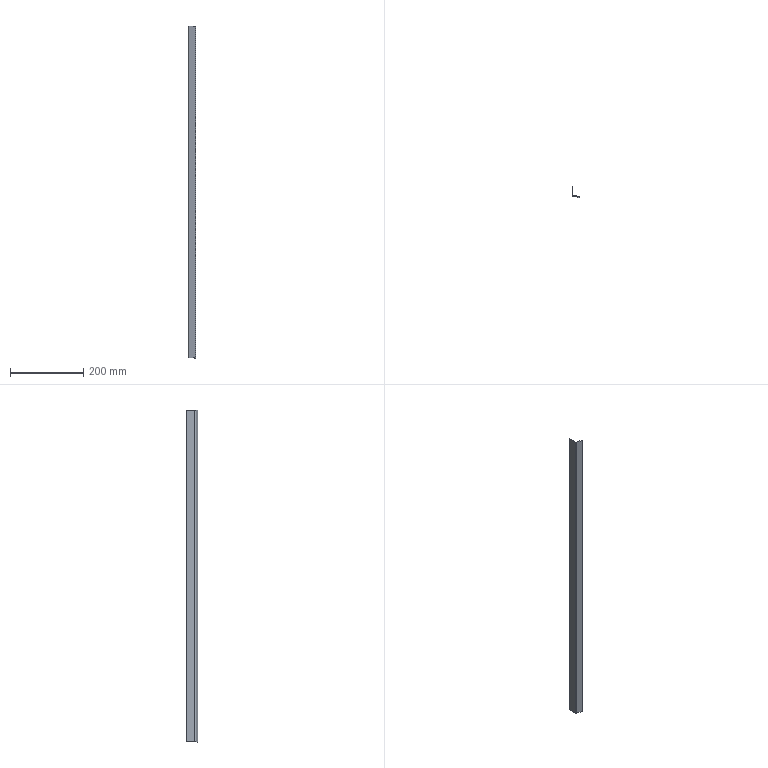Part | STEP file | 750078467 | 1 solid | 10 faces | box 19.629 x 30.176 x 903.6 mm | volume 47356 mm3 | plane 8 | cylinder 2 | commonest cylinder face diameters 2.4 x1 4.8 x1
STEP:
#1=CARTESIAN_POINT('',(0.,1.842,451.8));
#2=VERTEX_POINT('',#1);
#3=CARTESIAN_POINT('',(0.,25.,451.8));
#4=VERTEX_POINT('',#3);
#5=CARTESIAN_POINT('',(0.,0.,451.8));
#6=DIRECTION('',(0.,1.,0.));
#7=VECTOR('',#6,1000.);
#8=LINE('',#5,#7);
#9=EDGE_CURVE('',#2,#4,#8,.T.);
#10=ORIENTED_EDGE('',*,*,#9,.T.);
#11=CARTESIAN_POINT('',(0.,25.,-451.8));
#12=VERTEX_POINT('',#11);
#13=CARTESIAN_POINT('',(0.,25.,451.8));
#14=DIRECTION('',(0.,0.,-1.));
#15=VECTOR('',#14,1000.);
#16=LINE('',#13,#15);
#17=EDGE_CURVE('',#4,#12,#16,.T.);
#18=ORIENTED_EDGE('',*,*,#17,.T.);
#19=CARTESIAN_POINT('',(0.,1.842,-451.8));
#20=VERTEX_POINT('',#19);
#21=CARTESIAN_POINT('',(0.,0.,-451.8));
#22=DIRECTION('',(0.,-1.,0.));
#23=VECTOR('',#22,1000.);
#24=LINE('',#21,#23);
#25=EDGE_CURVE('',#12,#20,#24,.T.);
#26=ORIENTED_EDGE('',*,*,#25,.T.);
#27=CARTESIAN_POINT('',(0.,1.842,451.8));
#28=DIRECTION('',(0.,0.,1.));
#29=VECTOR('',#28,1000.);
#30=LINE('',#27,#29);
#31=EDGE_CURVE('',#20,#2,#30,.T.);
#32=ORIENTED_EDGE('',*,*,#31,.T.);
#33=EDGE_LOOP('',(#10,#18,#26,#32));
#34=FACE_OUTER_BOUND('',#33,.T.);
#35=CARTESIAN_POINT('',(0.,0.,451.8));
#36=DIRECTION('',(-1.,0.,0.));
#37=DIRECTION('',(0.,0.,1.));
#38=AXIS2_PLACEMENT_3D('',#35,#36,#37);
#39=PLANE('',#38);
#40=ADVANCED_FACE('',(#34),#39,.T.);
#41=CARTESIAN_POINT('',(1.2,25.,-451.8));
#42=VERTEX_POINT('',#41);
#43=CARTESIAN_POINT('',(0.,25.,-451.8));
#44=DIRECTION('',(-1.,0.,0.));
#45=VECTOR('',#44,1000.);
#46=LINE('',#43,#45);
#47=EDGE_CURVE('',#42,#12,#46,.T.);
#48=ORIENTED_EDGE('',*,*,#47,.T.);
#49=ORIENTED_EDGE('',*,*,#17,.F.);
#50=CARTESIAN_POINT('',(1.2,25.,451.8));
#51=VERTEX_POINT('',#50);
#52=CARTESIAN_POINT('',(0.,25.,451.8));
#53=DIRECTION('',(1.,0.,0.));
#54=VECTOR('',#53,1000.);
#55=LINE('',#52,#54);
#56=EDGE_CURVE('',#4,#51,#55,.T.);
#57=ORIENTED_EDGE('',*,*,#56,.T.);
#58=CARTESIAN_POINT('',(1.2,25.,451.8));
#59=DIRECTION('',(0.,0.,-1.));
#60=VECTOR('',#59,1000.);
#61=LINE('',#58,#60);
#62=EDGE_CURVE('',#51,#42,#61,.T.);
#63=ORIENTED_EDGE('',*,*,#62,.T.);
#64=EDGE_LOOP('',(#48,#49,#57,#63));
#65=FACE_OUTER_BOUND('',#64,.T.);
#66=CARTESIAN_POINT('',(0.,25.,451.8));
#67=DIRECTION('',(0.,1.,0.));
#68=DIRECTION('',(0.,0.,1.));
#69=AXIS2_PLACEMENT_3D('',#66,#67,#68);
#70=PLANE('',#69);
#71=ADVANCED_FACE('',(#65),#70,.T.);
#72=CARTESIAN_POINT('',(1.2,1.842,451.8));
#73=VERTEX_POINT('',#72);
#74=CARTESIAN_POINT('',(1.2,0.,451.8));
#75=DIRECTION('',(0.,1.,0.));
#76=VECTOR('',#75,1000.);
#77=LINE('',#74,#76);
#78=EDGE_CURVE('',#73,#51,#77,.T.);
#79=ORIENTED_EDGE('',*,*,#78,.T.);
#80=ORIENTED_EDGE('',*,*,#56,.F.);
#81=ORIENTED_EDGE('',*,*,#9,.F.);
#82=CARTESIAN_POINT('',(1.779,-0.4766,451.8));
#83=VERTEX_POINT('',#82);
#84=CARTESIAN_POINT('',(2.4,1.842,451.8));
#85=DIRECTION('',(0.,0.,1.));
#86=DIRECTION('',(-1.,0.,0.));
#87=AXIS2_PLACEMENT_3D('',#84,#85,#86);
#88=CIRCLE('',#87,2.4);
#89=EDGE_CURVE('',#2,#83,#88,.T.);
#90=ORIENTED_EDGE('',*,*,#89,.T.);
#91=CARTESIAN_POINT('',(19.319,-5.176,451.8));
#92=VERTEX_POINT('',#91);
#93=CARTESIAN_POINT('',(1.779,-0.4766,451.8));
#94=DIRECTION('',(0.9659,-0.2588,0.));
#95=VECTOR('',#94,1000.);
#96=LINE('',#93,#95);
#97=EDGE_CURVE('',#83,#92,#96,.T.);
#98=ORIENTED_EDGE('',*,*,#97,.T.);
#99=CARTESIAN_POINT('',(19.629,-4.017,451.8));
#100=VERTEX_POINT('',#99);
#101=CARTESIAN_POINT('',(19.319,-5.176,451.8));
#102=DIRECTION('',(0.2588,0.9659,0.));
#103=VECTOR('',#102,1000.);
#104=LINE('',#101,#103);
#105=EDGE_CURVE('',#92,#100,#104,.T.);
#106=ORIENTED_EDGE('',*,*,#105,.T.);
#107=CARTESIAN_POINT('',(2.089,0.6825,451.8));
#108=VERTEX_POINT('',#107);
#109=CARTESIAN_POINT('',(19.629,-4.017,451.8));
#110=DIRECTION('',(-0.9659,0.2588,0.));
#111=VECTOR('',#110,1000.);
#112=LINE('',#109,#111);
#113=EDGE_CURVE('',#100,#108,#112,.T.);
#114=ORIENTED_EDGE('',*,*,#113,.T.);
#115=CARTESIAN_POINT('',(2.4,1.842,451.8));
#116=DIRECTION('',(0.,0.,-1.));
#117=DIRECTION('',(-1.,0.,0.));
#118=AXIS2_PLACEMENT_3D('',#115,#116,#117);
#119=CIRCLE('',#118,1.2);
#120=EDGE_CURVE('',#108,#73,#119,.T.);
#121=ORIENTED_EDGE('',*,*,#120,.T.);
#122=EDGE_LOOP('',(#79,#80,#81,#90,#98,#106,#114,#121));
#123=FACE_OUTER_BOUND('',#122,.T.);
#124=CARTESIAN_POINT('',(0.,0.,451.8));
#125=DIRECTION('',(0.,0.,1.));
#126=DIRECTION('',(1.,0.,0.));
#127=AXIS2_PLACEMENT_3D('',#124,#125,#126);
#128=PLANE('',#127);
#129=ADVANCED_FACE('',(#123),#128,.T.);
#130=ORIENTED_EDGE('',*,*,#89,.F.);
#131=ORIENTED_EDGE('',*,*,#31,.F.);
#132=CARTESIAN_POINT('',(1.779,-0.4766,-451.8));
#133=VERTEX_POINT('',#132);
#134=CARTESIAN_POINT('',(2.4,1.842,-451.8));
#135=DIRECTION('',(0.,0.,1.));
#136=DIRECTION('',(-1.,0.,0.));
#137=AXIS2_PLACEMENT_3D('',#134,#135,#136);
#138=CIRCLE('',#137,2.4);
#139=EDGE_CURVE('',#20,#133,#138,.T.);
#140=ORIENTED_EDGE('',*,*,#139,.T.);
#141=CARTESIAN_POINT('',(1.779,-0.4766,451.8));
#142=DIRECTION('',(0.,0.,1.));
#143=VECTOR('',#142,1000.);
#144=LINE('',#141,#143);
#145=EDGE_CURVE('',#133,#83,#144,.T.);
#146=ORIENTED_EDGE('',*,*,#145,.T.);
#147=EDGE_LOOP('',(#130,#131,#140,#146));
#148=FACE_OUTER_BOUND('',#147,.T.);
#149=CARTESIAN_POINT('',(2.4,1.842,451.8));
#150=DIRECTION('',(0.,0.,-1.));
#151=DIRECTION('',(-1.,0.,0.));
#152=AXIS2_PLACEMENT_3D('',#149,#150,#151);
#153=CYLINDRICAL_SURFACE('',#152,2.4);
#154=ADVANCED_FACE('',(#148),#153,.T.);
#155=ORIENTED_EDGE('',*,*,#139,.F.);
#156=ORIENTED_EDGE('',*,*,#25,.F.);
#157=ORIENTED_EDGE('',*,*,#47,.F.);
#158=CARTESIAN_POINT('',(1.2,1.842,-451.8));
#159=VERTEX_POINT('',#158);
#160=CARTESIAN_POINT('',(1.2,-5.176,-451.8));
#161=DIRECTION('',(0.,1.,0.));
#162=VECTOR('',#161,1000.);
#163=LINE('',#160,#162);
#164=EDGE_CURVE('',#159,#42,#163,.T.);
#165=ORIENTED_EDGE('',*,*,#164,.F.);
#166=CARTESIAN_POINT('',(2.089,0.6825,-451.8));
#167=VERTEX_POINT('',#166);
#168=CARTESIAN_POINT('',(2.4,1.842,-451.8));
#169=DIRECTION('',(0.,0.,1.));
#170=DIRECTION('',(-1.,0.,0.));
#171=AXIS2_PLACEMENT_3D('',#168,#169,#170);
#172=CIRCLE('',#171,1.2);
#173=EDGE_CURVE('',#159,#167,#172,.T.);
#174=ORIENTED_EDGE('',*,*,#173,.T.);
#175=CARTESIAN_POINT('',(19.629,-4.017,-451.8));
#176=VERTEX_POINT('',#175);
#177=CARTESIAN_POINT('',(19.629,-4.017,-451.8));
#178=DIRECTION('',(-0.9659,0.2588,0.));
#179=VECTOR('',#178,1000.);
#180=LINE('',#177,#179);
#181=EDGE_CURVE('',#176,#167,#180,.T.);
#182=ORIENTED_EDGE('',*,*,#181,.F.);
#183=CARTESIAN_POINT('',(19.319,-5.176,-451.8));
#184=VERTEX_POINT('',#183);
#185=CARTESIAN_POINT('',(19.319,-5.176,-451.8));
#186=DIRECTION('',(-0.2588,-0.9659,0.));
#187=VECTOR('',#186,1000.);
#188=LINE('',#185,#187);
#189=EDGE_CURVE('',#176,#184,#188,.T.);
#190=ORIENTED_EDGE('',*,*,#189,.T.);
#191=CARTESIAN_POINT('',(1.779,-0.4766,-451.8));
#192=DIRECTION('',(0.9659,-0.2588,0.));
#193=VECTOR('',#192,1000.);
#194=LINE('',#191,#193);
#195=EDGE_CURVE('',#133,#184,#194,.T.);
#196=ORIENTED_EDGE('',*,*,#195,.F.);
#197=EDGE_LOOP('',(#155,#156,#157,#165,#174,#182,#190,#196));
#198=FACE_OUTER_BOUND('',#197,.T.);
#199=CARTESIAN_POINT('',(19.319,-5.176,-451.8));
#200=DIRECTION('',(0.,0.,1.));
#201=DIRECTION('',(1.,0.,0.));
#202=AXIS2_PLACEMENT_3D('',#199,#200,#201);
#203=PLANE('',#202);
#204=ADVANCED_FACE('',(#198),#203,.F.);
#205=ORIENTED_EDGE('',*,*,#62,.F.);
#206=ORIENTED_EDGE('',*,*,#78,.F.);
#207=CARTESIAN_POINT('',(1.2,1.842,451.8));
#208=DIRECTION('',(0.,0.,1.));
#209=VECTOR('',#208,1000.);
#210=LINE('',#207,#209);
#211=EDGE_CURVE('',#159,#73,#210,.T.);
#212=ORIENTED_EDGE('',*,*,#211,.F.);
#213=ORIENTED_EDGE('',*,*,#164,.T.);
#214=EDGE_LOOP('',(#205,#206,#212,#213));
#215=FACE_OUTER_BOUND('',#214,.T.);
#216=CARTESIAN_POINT('',(1.2,0.,451.8));
#217=DIRECTION('',(-1.,0.,0.));
#218=DIRECTION('',(0.,0.,1.));
#219=AXIS2_PLACEMENT_3D('',#216,#217,#218);
#220=PLANE('',#219);
#221=ADVANCED_FACE('',(#215),#220,.F.);
#222=CARTESIAN_POINT('',(2.089,0.6825,451.8));
#223=DIRECTION('',(0.,0.,-1.));
#224=VECTOR('',#223,1000.);
#225=LINE('',#222,#224);
#226=EDGE_CURVE('',#108,#167,#225,.T.);
#227=ORIENTED_EDGE('',*,*,#226,.F.);
#228=ORIENTED_EDGE('',*,*,#113,.F.);
#229=CARTESIAN_POINT('',(19.629,-4.017,451.8));
#230=DIRECTION('',(0.,0.,1.));
#231=VECTOR('',#230,1000.);
#232=LINE('',#229,#231);
#233=EDGE_CURVE('',#176,#100,#232,.T.);
#234=ORIENTED_EDGE('',*,*,#233,.F.);
#235=ORIENTED_EDGE('',*,*,#181,.T.);
#236=EDGE_LOOP('',(#227,#228,#234,#235));
#237=FACE_OUTER_BOUND('',#236,.T.);
#238=CARTESIAN_POINT('',(19.629,-4.017,451.8));
#239=DIRECTION('',(-0.2588,-0.9659,0.));
#240=DIRECTION('',(0.9659,-0.2588,0.));
#241=AXIS2_PLACEMENT_3D('',#238,#239,#240);
#242=PLANE('',#241);
#243=ADVANCED_FACE('',(#237),#242,.F.);
#244=ORIENTED_EDGE('',*,*,#97,.F.);
#245=ORIENTED_EDGE('',*,*,#145,.F.);
#246=ORIENTED_EDGE('',*,*,#195,.T.);
#247=CARTESIAN_POINT('',(19.319,-5.176,451.8));
#248=DIRECTION('',(0.,0.,1.));
#249=VECTOR('',#248,1000.);
#250=LINE('',#247,#249);
#251=EDGE_CURVE('',#184,#92,#250,.T.);
#252=ORIENTED_EDGE('',*,*,#251,.T.);
#253=EDGE_LOOP('',(#244,#245,#246,#252));
#254=FACE_OUTER_BOUND('',#253,.T.);
#255=CARTESIAN_POINT('',(19.319,-5.176,451.8));
#256=DIRECTION('',(-0.2588,-0.9659,0.));
#257=DIRECTION('',(0.9659,-0.2588,0.));
#258=AXIS2_PLACEMENT_3D('',#255,#256,#257);
#259=PLANE('',#258);
#260=ADVANCED_FACE('',(#254),#259,.T.);
#261=ORIENTED_EDGE('',*,*,#211,.T.);
#262=ORIENTED_EDGE('',*,*,#120,.F.);
#263=ORIENTED_EDGE('',*,*,#226,.T.);
#264=ORIENTED_EDGE('',*,*,#173,.F.);
#265=EDGE_LOOP('',(#261,#262,#263,#264));
#266=FACE_OUTER_BOUND('',#265,.T.);
#267=CARTESIAN_POINT('',(2.4,1.842,451.8));
#268=DIRECTION('',(0.,0.,-1.));
#269=DIRECTION('',(-1.,0.,0.));
#270=AXIS2_PLACEMENT_3D('',#267,#268,#269);
#271=CYLINDRICAL_SURFACE('',#270,1.2);
#272=ADVANCED_FACE('',(#266),#271,.F.);
#273=ORIENTED_EDGE('',*,*,#105,.F.);
#274=ORIENTED_EDGE('',*,*,#251,.F.);
#275=ORIENTED_EDGE('',*,*,#189,.F.);
#276=ORIENTED_EDGE('',*,*,#233,.T.);
#277=EDGE_LOOP('',(#273,#274,#275,#276));
#278=FACE_OUTER_BOUND('',#277,.T.);
#279=CARTESIAN_POINT('',(19.319,-5.176,451.8));
#280=DIRECTION('',(-0.9659,0.2588,0.));
#281=DIRECTION('',(-0.2588,-0.9659,0.));
#282=AXIS2_PLACEMENT_3D('',#279,#280,#281);
#283=PLANE('',#282);
#284=ADVANCED_FACE('',(#278),#283,.F.);
#285=CLOSED_SHELL('',(#40,#71,#129,#154,#204,#221,#243,#260,#272,#284));
#286=MANIFOLD_SOLID_BREP('',#285);
#287=CARTESIAN_POINT('',(0.,0.,0.));
#288=DIRECTION('',(0.,0.,1.));
#289=DIRECTION('',(1.,0.,0.));
#290=AXIS2_PLACEMENT_3D('',#287,#288,#289);
#291=(LENGTH_UNIT()NAMED_UNIT(*)SI_UNIT(.MILLI.,.METRE.));
#292=UNCERTAINTY_MEASURE_WITH_UNIT(LENGTH_MEASURE(0.00001),#291,'','');
#293=(NAMED_UNIT(*)PLANE_ANGLE_UNIT()SI_UNIT($,.RADIAN.));
#294=(NAMED_UNIT(*)SI_UNIT($,.STERADIAN.)SOLID_ANGLE_UNIT());
#295=(GEOMETRIC_REPRESENTATION_CONTEXT(3)GLOBAL_UNCERTAINTY_ASSIGNED_CONTEXT((#292))GLOBAL_UNIT_ASSIGNED_CONTEXT((#291,#293,#294))REPRESENTATION_CONTEXT('',''));
#296=ADVANCED_BREP_SHAPE_REPRESENTATION('',(#286,#290),#295);